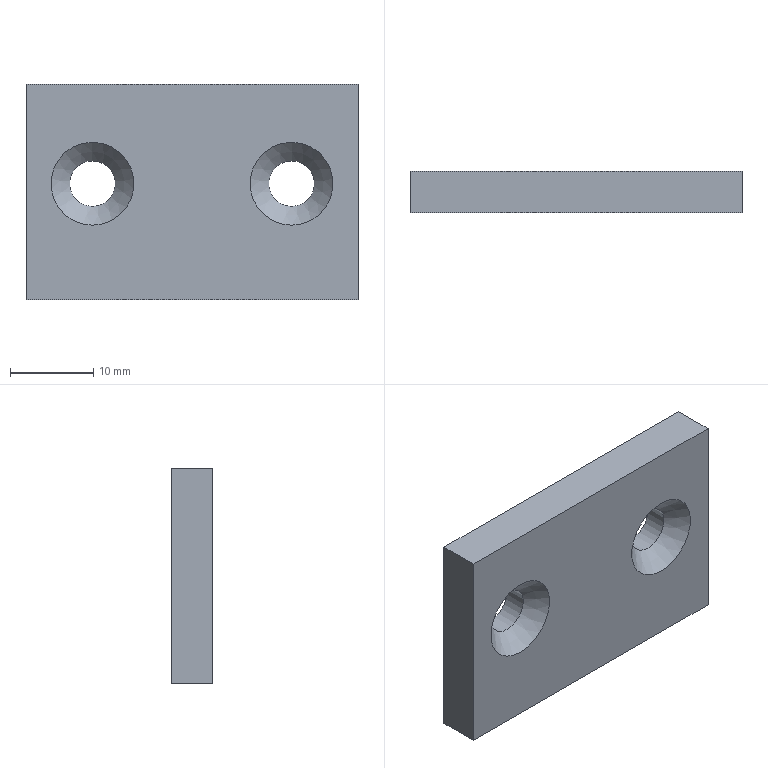Part | NX | features DATUM_CSYS 3, CSUNK_HOLE 2, SKETCH 2, EXTRUDE 1, HOLE PACKAGE 1 | 1 solid | 10 faces | box 40 x 5 x 26 mm | volume 4851 mm3 | plane 6 | cylinder 2 | cone 2 | commonest cylinder face diameters 5.5 x2
STEP:
#1=CARTESIAN_POINT('',(-20.,0.,26.));
#2=VERTEX_POINT('',#1);
#3=CARTESIAN_POINT('',(-20.,0.,0.));
#4=VERTEX_POINT('',#3);
#5=CARTESIAN_POINT('',(-20.,0.,26.));
#6=DIRECTION('',(0.,0.,-1.));
#7=VECTOR('',#6,1000.);
#8=LINE('',#5,#7);
#9=EDGE_CURVE('',#2,#4,#8,.T.);
#10=ORIENTED_EDGE('',*,*,#9,.F.);
#11=CARTESIAN_POINT('',(-20.,5.,26.));
#12=VERTEX_POINT('',#11);
#13=CARTESIAN_POINT('',(-20.,5.,26.));
#14=DIRECTION('',(0.,-1.,0.));
#15=VECTOR('',#14,1000.);
#16=LINE('',#13,#15);
#17=EDGE_CURVE('',#12,#2,#16,.T.);
#18=ORIENTED_EDGE('',*,*,#17,.F.);
#19=CARTESIAN_POINT('',(-20.,5.,0.));
#20=VERTEX_POINT('',#19);
#21=CARTESIAN_POINT('',(-20.,5.,26.));
#22=DIRECTION('',(0.,0.,-1.));
#23=VECTOR('',#22,1000.);
#24=LINE('',#21,#23);
#25=EDGE_CURVE('',#12,#20,#24,.T.);
#26=ORIENTED_EDGE('',*,*,#25,.T.);
#27=CARTESIAN_POINT('',(-20.,5.,0.));
#28=DIRECTION('',(0.,-1.,0.));
#29=VECTOR('',#28,1000.);
#30=LINE('',#27,#29);
#31=EDGE_CURVE('',#20,#4,#30,.T.);
#32=ORIENTED_EDGE('',*,*,#31,.T.);
#33=EDGE_LOOP('',(#10,#18,#26,#32));
#34=FACE_BOUND('',#33,.T.);
#35=CARTESIAN_POINT('',(-20.,5.,26.));
#36=DIRECTION('',(-1.,0.,0.));
#37=DIRECTION('',(0.,0.,1.));
#38=AXIS2_PLACEMENT_3D('',#35,#36,#37);
#39=PLANE('',#38);
#40=ADVANCED_FACE('',(#34),#39,.T.);
#41=CARTESIAN_POINT('',(20.,0.,0.));
#42=VERTEX_POINT('',#41);
#43=CARTESIAN_POINT('',(-20.,0.,0.));
#44=DIRECTION('',(1.,0.,0.));
#45=VECTOR('',#44,1000.);
#46=LINE('',#43,#45);
#47=EDGE_CURVE('',#4,#42,#46,.T.);
#48=ORIENTED_EDGE('',*,*,#47,.F.);
#49=ORIENTED_EDGE('',*,*,#31,.F.);
#50=CARTESIAN_POINT('',(20.,5.,0.));
#51=VERTEX_POINT('',#50);
#52=CARTESIAN_POINT('',(-20.,5.,0.));
#53=DIRECTION('',(1.,0.,0.));
#54=VECTOR('',#53,1000.);
#55=LINE('',#52,#54);
#56=EDGE_CURVE('',#20,#51,#55,.T.);
#57=ORIENTED_EDGE('',*,*,#56,.T.);
#58=CARTESIAN_POINT('',(20.,5.,0.));
#59=DIRECTION('',(0.,-1.,0.));
#60=VECTOR('',#59,1000.);
#61=LINE('',#58,#60);
#62=EDGE_CURVE('',#51,#42,#61,.T.);
#63=ORIENTED_EDGE('',*,*,#62,.T.);
#64=EDGE_LOOP('',(#48,#49,#57,#63));
#65=FACE_BOUND('',#64,.T.);
#66=CARTESIAN_POINT('',(-20.,5.,0.));
#67=DIRECTION('',(0.,0.,-1.));
#68=DIRECTION('',(-1.,0.,0.));
#69=AXIS2_PLACEMENT_3D('',#66,#67,#68);
#70=PLANE('',#69);
#71=ADVANCED_FACE('',(#65),#70,.T.);
#72=CARTESIAN_POINT('',(20.,0.,26.));
#73=VERTEX_POINT('',#72);
#74=CARTESIAN_POINT('',(20.,0.,0.));
#75=DIRECTION('',(0.,0.,1.));
#76=VECTOR('',#75,1000.);
#77=LINE('',#74,#76);
#78=EDGE_CURVE('',#42,#73,#77,.T.);
#79=ORIENTED_EDGE('',*,*,#78,.F.);
#80=ORIENTED_EDGE('',*,*,#62,.F.);
#81=CARTESIAN_POINT('',(20.,5.,26.));
#82=VERTEX_POINT('',#81);
#83=CARTESIAN_POINT('',(20.,5.,0.));
#84=DIRECTION('',(0.,0.,1.));
#85=VECTOR('',#84,1000.);
#86=LINE('',#83,#85);
#87=EDGE_CURVE('',#51,#82,#86,.T.);
#88=ORIENTED_EDGE('',*,*,#87,.T.);
#89=CARTESIAN_POINT('',(20.,5.,26.));
#90=DIRECTION('',(0.,-1.,0.));
#91=VECTOR('',#90,1000.);
#92=LINE('',#89,#91);
#93=EDGE_CURVE('',#82,#73,#92,.T.);
#94=ORIENTED_EDGE('',*,*,#93,.T.);
#95=EDGE_LOOP('',(#79,#80,#88,#94));
#96=FACE_BOUND('',#95,.T.);
#97=CARTESIAN_POINT('',(20.,5.,0.));
#98=DIRECTION('',(1.,0.,0.));
#99=DIRECTION('',(0.,0.,-1.));
#100=AXIS2_PLACEMENT_3D('',#97,#98,#99);
#101=PLANE('',#100);
#102=ADVANCED_FACE('',(#96),#101,.T.);
#103=CARTESIAN_POINT('',(20.,0.,26.));
#104=DIRECTION('',(-1.,0.,0.));
#105=VECTOR('',#104,1000.);
#106=LINE('',#103,#105);
#107=EDGE_CURVE('',#73,#2,#106,.T.);
#108=ORIENTED_EDGE('',*,*,#107,.F.);
#109=ORIENTED_EDGE('',*,*,#93,.F.);
#110=CARTESIAN_POINT('',(20.,5.,26.));
#111=DIRECTION('',(-1.,0.,0.));
#112=VECTOR('',#111,1000.);
#113=LINE('',#110,#112);
#114=EDGE_CURVE('',#82,#12,#113,.T.);
#115=ORIENTED_EDGE('',*,*,#114,.T.);
#116=ORIENTED_EDGE('',*,*,#17,.T.);
#117=EDGE_LOOP('',(#108,#109,#115,#116));
#118=FACE_BOUND('',#117,.T.);
#119=CARTESIAN_POINT('',(20.,5.,26.));
#120=DIRECTION('',(0.,0.,1.));
#121=DIRECTION('',(1.,0.,0.));
#122=AXIS2_PLACEMENT_3D('',#119,#120,#121);
#123=PLANE('',#122);
#124=ADVANCED_FACE('',(#118),#123,.T.);
#125=CARTESIAN_POINT('',(12.,5.,11.25));
#126=VERTEX_POINT('',#125);
#127=CARTESIAN_POINT('',(12.,5.,14.));
#128=DIRECTION('',(0.,-1.,0.));
#129=DIRECTION('',(0.,0.,-1.));
#130=AXIS2_PLACEMENT_3D('',#127,#128,#129);
#131=CIRCLE('',#130,2.75);
#132=EDGE_CURVE('',#126,#126,#131,.T.);
#133=ORIENTED_EDGE('',*,*,#132,.T.);
#134=EDGE_LOOP('',(#133));
#135=FACE_BOUND('',#134,.T.);
#136=CARTESIAN_POINT('',(-12.,5.,11.25));
#137=VERTEX_POINT('',#136);
#138=CARTESIAN_POINT('',(-12.,5.,14.));
#139=DIRECTION('',(0.,-1.,0.));
#140=DIRECTION('',(0.,0.,-1.));
#141=AXIS2_PLACEMENT_3D('',#138,#139,#140);
#142=CIRCLE('',#141,2.75);
#143=EDGE_CURVE('',#137,#137,#142,.T.);
#144=ORIENTED_EDGE('',*,*,#143,.T.);
#145=EDGE_LOOP('',(#144));
#146=FACE_BOUND('',#145,.T.);
#147=ORIENTED_EDGE('',*,*,#25,.F.);
#148=ORIENTED_EDGE('',*,*,#114,.F.);
#149=ORIENTED_EDGE('',*,*,#87,.F.);
#150=ORIENTED_EDGE('',*,*,#56,.F.);
#151=EDGE_LOOP('',(#147,#148,#149,#150));
#152=FACE_BOUND('',#151,.T.);
#153=CARTESIAN_POINT('',(0.,5.,0.));
#154=DIRECTION('',(0.,-1.,0.));
#155=DIRECTION('',(0.,0.,-1.));
#156=AXIS2_PLACEMENT_3D('',#153,#154,#155);
#157=PLANE('',#156);
#158=ADVANCED_FACE('',(#135,#146,#152),#157,.F.);
#159=CARTESIAN_POINT('',(12.,0.,19.));
#160=VERTEX_POINT('',#159);
#161=CARTESIAN_POINT('',(12.,0.,14.));
#162=DIRECTION('',(0.,1.,0.));
#163=DIRECTION('',(0.,0.,1.));
#164=AXIS2_PLACEMENT_3D('',#161,#162,#163);
#165=CIRCLE('',#164,5.);
#166=EDGE_CURVE('',#160,#160,#165,.T.);
#167=ORIENTED_EDGE('',*,*,#166,.T.);
#168=EDGE_LOOP('',(#167));
#169=FACE_BOUND('',#168,.T.);
#170=CARTESIAN_POINT('',(-12.,0.,19.));
#171=VERTEX_POINT('',#170);
#172=CARTESIAN_POINT('',(-12.,0.,14.));
#173=DIRECTION('',(0.,1.,0.));
#174=DIRECTION('',(0.,0.,1.));
#175=AXIS2_PLACEMENT_3D('',#172,#173,#174);
#176=CIRCLE('',#175,5.);
#177=EDGE_CURVE('',#171,#171,#176,.T.);
#178=ORIENTED_EDGE('',*,*,#177,.T.);
#179=EDGE_LOOP('',(#178));
#180=FACE_BOUND('',#179,.T.);
#181=ORIENTED_EDGE('',*,*,#9,.T.);
#182=ORIENTED_EDGE('',*,*,#47,.T.);
#183=ORIENTED_EDGE('',*,*,#78,.T.);
#184=ORIENTED_EDGE('',*,*,#107,.T.);
#185=EDGE_LOOP('',(#181,#182,#183,#184));
#186=FACE_BOUND('',#185,.T.);
#187=CARTESIAN_POINT('',(0.,0.,0.));
#188=DIRECTION('',(0.,-1.,0.));
#189=DIRECTION('',(0.,0.,-1.));
#190=AXIS2_PLACEMENT_3D('',#187,#188,#189);
#191=PLANE('',#190);
#192=ADVANCED_FACE('',(#169,#180,#186),#191,.T.);
#193=CARTESIAN_POINT('',(-12.,2.25,16.75));
#194=VERTEX_POINT('',#193);
#195=CARTESIAN_POINT('',(-12.,2.25,14.));
#196=DIRECTION('',(0.,1.,0.));
#197=DIRECTION('',(0.,0.,1.));
#198=AXIS2_PLACEMENT_3D('',#195,#196,#197);
#199=CIRCLE('',#198,2.75);
#200=EDGE_CURVE('',#194,#194,#199,.F.);
#201=ORIENTED_EDGE('',*,*,#200,.T.);
#202=EDGE_LOOP('',(#201));
#203=FACE_BOUND('',#202,.T.);
#204=ORIENTED_EDGE('',*,*,#143,.F.);
#205=EDGE_LOOP('',(#204));
#206=FACE_BOUND('',#205,.T.);
#207=CARTESIAN_POINT('',(-12.,25.975,14.));
#208=DIRECTION('',(0.,1.,0.));
#209=DIRECTION('',(0.,0.,1.));
#210=AXIS2_PLACEMENT_3D('',#207,#208,#209);
#211=CYLINDRICAL_SURFACE('',#210,2.75);
#212=ADVANCED_FACE('',(#203,#206),#211,.F.);
#213=ORIENTED_EDGE('',*,*,#200,.F.);
#214=EDGE_LOOP('',(#213));
#215=FACE_BOUND('',#214,.T.);
#216=ORIENTED_EDGE('',*,*,#177,.F.);
#217=EDGE_LOOP('',(#216));
#218=FACE_BOUND('',#217,.T.);
#219=CARTESIAN_POINT('',(-12.,0.,14.));
#220=DIRECTION('',(0.,-1.,0.));
#221=DIRECTION('',(0.,0.,-1.));
#222=AXIS2_PLACEMENT_3D('',#219,#220,#221);
#223=CONICAL_SURFACE('',#222,5.,0.7854);
#224=ADVANCED_FACE('',(#215,#218),#223,.F.);
#225=CARTESIAN_POINT('',(12.,2.25,16.75));
#226=VERTEX_POINT('',#225);
#227=CARTESIAN_POINT('',(12.,2.25,14.));
#228=DIRECTION('',(0.,1.,0.));
#229=DIRECTION('',(0.,0.,1.));
#230=AXIS2_PLACEMENT_3D('',#227,#228,#229);
#231=CIRCLE('',#230,2.75);
#232=EDGE_CURVE('',#226,#226,#231,.F.);
#233=ORIENTED_EDGE('',*,*,#232,.T.);
#234=EDGE_LOOP('',(#233));
#235=FACE_BOUND('',#234,.T.);
#236=ORIENTED_EDGE('',*,*,#132,.F.);
#237=EDGE_LOOP('',(#236));
#238=FACE_BOUND('',#237,.T.);
#239=CARTESIAN_POINT('',(12.,25.975,14.));
#240=DIRECTION('',(0.,1.,0.));
#241=DIRECTION('',(0.,0.,1.));
#242=AXIS2_PLACEMENT_3D('',#239,#240,#241);
#243=CYLINDRICAL_SURFACE('',#242,2.75);
#244=ADVANCED_FACE('',(#235,#238),#243,.F.);
#245=ORIENTED_EDGE('',*,*,#232,.F.);
#246=EDGE_LOOP('',(#245));
#247=FACE_BOUND('',#246,.T.);
#248=ORIENTED_EDGE('',*,*,#166,.F.);
#249=EDGE_LOOP('',(#248));
#250=FACE_BOUND('',#249,.T.);
#251=CARTESIAN_POINT('',(12.,0.,14.));
#252=DIRECTION('',(0.,-1.,0.));
#253=DIRECTION('',(0.,0.,-1.));
#254=AXIS2_PLACEMENT_3D('',#251,#252,#253);
#255=CONICAL_SURFACE('',#254,5.,0.7854);
#256=ADVANCED_FACE('',(#247,#250),#255,.F.);
#257=CLOSED_SHELL('',(#40,#71,#102,#124,#158,#192,#212,#224,#244,#256));
#258=MANIFOLD_SOLID_BREP('',#257);
#259=(LENGTH_UNIT()NAMED_UNIT(*)SI_UNIT(.MILLI.,.METRE.));
#260=UNCERTAINTY_MEASURE_WITH_UNIT(LENGTH_MEASURE(0.00001),#259,'','');
#261=(NAMED_UNIT(*)PLANE_ANGLE_UNIT()SI_UNIT($,.RADIAN.));
#262=(NAMED_UNIT(*)SI_UNIT($,.STERADIAN.)SOLID_ANGLE_UNIT());
#263=(GEOMETRIC_REPRESENTATION_CONTEXT(3)GLOBAL_UNCERTAINTY_ASSIGNED_CONTEXT((#260))GLOBAL_UNIT_ASSIGNED_CONTEXT((#259,#261,#262))REPRESENTATION_CONTEXT('',''));
#264=ADVANCED_BREP_SHAPE_REPRESENTATION('',(#258),#263);